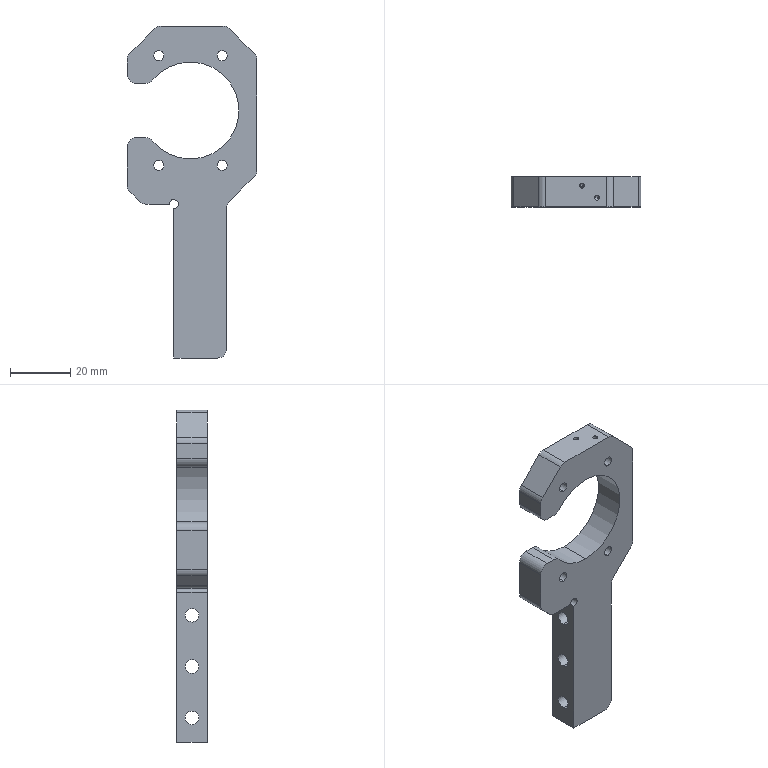Part | STEP file | PN_0007 | 1 solid | 65 faces | box 43 x 10 x 110 mm | volume 21722 mm3 | cylinder 42 | plane 19 | cone 4 | commonest cylinder face diameters 6 x13 3.3 x8 4.5 x6 8 x6 1.6 x4 32.1 x3